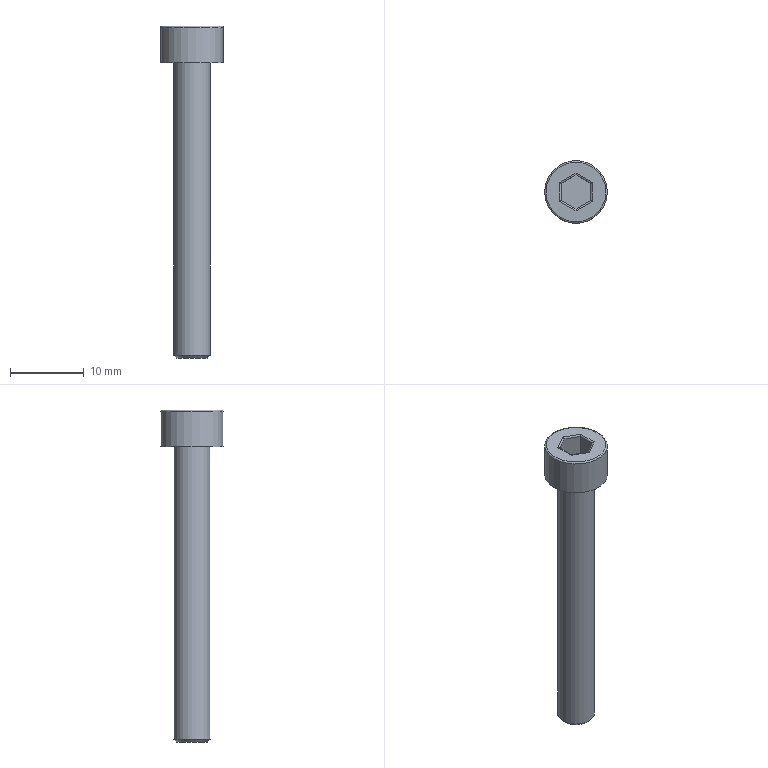Part | STEP file | 200 mesh_id694_x | 1 solid | 20 faces | box 8.5 x 8.5 x 45 mm | volume 1026 mm3 | plane 10 | cylinder 8 | torus 1 | cone 1 | commonest cylinder face diameters 0.4 x6 5 x1 8.5 x1
STEP:
#1=CARTESIAN_POINT('',(-17212.884,-3990.36,100.));
#2=VERTEX_POINT('',#1);
#3=CARTESIAN_POINT('',(-17215.084,-3989.089,100.));
#4=VERTEX_POINT('',#3);
#5=CARTESIAN_POINT('',(-17214.984,-3989.147,100.));
#6=DIRECTION('',(-0.866,0.5,0.));
#7=VECTOR('',#6,1.);
#8=LINE('',#5,#7);
#9=EDGE_CURVE('',#2,#4,#8,.T.);
#10=ORIENTED_EDGE('',*,*,#9,.T.);
#11=CARTESIAN_POINT('',(-17215.084,-3986.549,100.));
#12=VERTEX_POINT('',#11);
#13=CARTESIAN_POINT('',(-17215.084,-3986.664,100.));
#14=DIRECTION('',(0.,1.,0.));
#15=VECTOR('',#14,1.);
#16=LINE('',#13,#15);
#17=EDGE_CURVE('',#4,#12,#16,.T.);
#18=ORIENTED_EDGE('',*,*,#17,.T.);
#19=CARTESIAN_POINT('',(-17212.884,-3985.279,100.));
#20=VERTEX_POINT('',#19);
#21=CARTESIAN_POINT('',(-17212.984,-3985.337,100.));
#22=DIRECTION('',(0.866,0.5,0.));
#23=VECTOR('',#22,1.);
#24=LINE('',#21,#23);
#25=EDGE_CURVE('',#12,#20,#24,.T.);
#26=ORIENTED_EDGE('',*,*,#25,.T.);
#27=CARTESIAN_POINT('',(-17210.684,-3986.549,100.));
#28=VERTEX_POINT('',#27);
#29=CARTESIAN_POINT('',(-17210.784,-3986.491,100.));
#30=DIRECTION('',(0.866,-0.5,0.));
#31=VECTOR('',#30,1.);
#32=LINE('',#29,#31);
#33=EDGE_CURVE('',#20,#28,#32,.T.);
#34=ORIENTED_EDGE('',*,*,#33,.T.);
#35=CARTESIAN_POINT('',(-17210.684,-3989.089,100.));
#36=VERTEX_POINT('',#35);
#37=CARTESIAN_POINT('',(-17210.684,-3988.974,100.));
#38=DIRECTION('',(0.,-1.,0.));
#39=VECTOR('',#38,1.);
#40=LINE('',#37,#39);
#41=EDGE_CURVE('',#28,#36,#40,.T.);
#42=ORIENTED_EDGE('',*,*,#41,.T.);
#43=CARTESIAN_POINT('',(-17212.784,-3990.302,100.));
#44=DIRECTION('',(-0.866,-0.5,0.));
#45=VECTOR('',#44,1.);
#46=LINE('',#43,#45);
#47=EDGE_CURVE('',#36,#2,#46,.T.);
#48=ORIENTED_EDGE('',*,*,#47,.T.);
#49=EDGE_LOOP('',(#10,#18,#26,#34,#42,#48));
#50=FACE_BOUND('',#49,.T.);
#51=CARTESIAN_POINT('',(-17208.834,-3987.819,100.));
#52=VERTEX_POINT('',#51);
#53=CARTESIAN_POINT('',(-17212.884,-3987.819,100.));
#54=DIRECTION('',(0.,0.,1.));
#55=DIRECTION('',(1.,0.,0.));
#56=AXIS2_PLACEMENT_3D('',#53,#54,#55);
#57=CIRCLE('',#56,4.05);
#58=EDGE_CURVE('',#52,#52,#57,.T.);
#59=ORIENTED_EDGE('',*,*,#58,.T.);
#60=EDGE_LOOP('',(#59));
#61=FACE_BOUND('',#60,.T.);
#62=CARTESIAN_POINT('',(-17212.884,-3987.819,100.));
#63=DIRECTION('',(0.,0.,1.));
#64=DIRECTION('',(1.,0.,0.));
#65=AXIS2_PLACEMENT_3D('',#62,#63,#64);
#66=PLANE('',#65);
#67=ADVANCED_FACE('',(#50,#61),#66,.T.);
#68=CARTESIAN_POINT('',(-17215.384,-3987.819,95.));
#69=VERTEX_POINT('',#68);
#70=CARTESIAN_POINT('',(-17212.884,-3987.819,95.));
#71=DIRECTION('',(0.,0.,1.));
#72=DIRECTION('',(-1.,0.,0.));
#73=AXIS2_PLACEMENT_3D('',#70,#71,#72);
#74=CIRCLE('',#73,2.5);
#75=EDGE_CURVE('',#69,#69,#74,.T.);
#76=ORIENTED_EDGE('',*,*,#75,.T.);
#77=EDGE_LOOP('',(#76));
#78=FACE_BOUND('',#77,.T.);
#79=CARTESIAN_POINT('',(-17208.634,-3987.819,95.));
#80=VERTEX_POINT('',#79);
#81=CARTESIAN_POINT('',(-17212.884,-3987.819,95.));
#82=DIRECTION('',(0.,0.,1.));
#83=DIRECTION('',(1.,0.,0.));
#84=AXIS2_PLACEMENT_3D('',#81,#82,#83);
#85=CIRCLE('',#84,4.25);
#86=EDGE_CURVE('',#80,#80,#85,.T.);
#87=ORIENTED_EDGE('',*,*,#86,.F.);
#88=EDGE_LOOP('',(#87));
#89=FACE_BOUND('',#88,.T.);
#90=CARTESIAN_POINT('',(-17212.884,-3987.819,95.));
#91=DIRECTION('',(0.,0.,-1.));
#92=DIRECTION('',(-1.,0.,0.));
#93=AXIS2_PLACEMENT_3D('',#90,#91,#92);
#94=PLANE('',#93);
#95=ADVANCED_FACE('',(#78,#89),#94,.T.);
#96=CARTESIAN_POINT('',(-17208.634,-3987.819,99.8));
#97=VERTEX_POINT('',#96);
#98=CARTESIAN_POINT('',(-17212.884,-3987.819,99.8));
#99=DIRECTION('',(0.,0.,-1.));
#100=DIRECTION('',(1.,0.,0.));
#101=AXIS2_PLACEMENT_3D('',#98,#99,#100);
#102=CIRCLE('',#101,4.25);
#103=EDGE_CURVE('',#97,#97,#102,.T.);
#104=ORIENTED_EDGE('',*,*,#103,.T.);
#105=EDGE_LOOP('',(#104));
#106=FACE_BOUND('',#105,.T.);
#107=ORIENTED_EDGE('',*,*,#86,.T.);
#108=EDGE_LOOP('',(#107));
#109=FACE_BOUND('',#108,.T.);
#110=CARTESIAN_POINT('',(-17212.884,-3987.819,95.));
#111=DIRECTION('',(0.,0.,1.));
#112=DIRECTION('',(1.,0.,0.));
#113=AXIS2_PLACEMENT_3D('',#110,#111,#112);
#114=CYLINDRICAL_SURFACE('',#113,4.25);
#115=ADVANCED_FACE('',(#106,#109),#114,.T.);
#116=ORIENTED_EDGE('',*,*,#58,.F.);
#117=EDGE_LOOP('',(#116));
#118=FACE_BOUND('',#117,.T.);
#119=ORIENTED_EDGE('',*,*,#103,.F.);
#120=EDGE_LOOP('',(#119));
#121=FACE_BOUND('',#120,.T.);
#122=CARTESIAN_POINT('',(-17212.884,-3987.819,99.8));
#123=DIRECTION('',(0.,0.,1.));
#124=DIRECTION('',(1.,0.,0.));
#125=AXIS2_PLACEMENT_3D('',#122,#123,#124);
#126=TOROIDAL_SURFACE('',#125,4.05,0.2);
#127=ADVANCED_FACE('',(#118,#121),#126,.T.);
#128=CARTESIAN_POINT('',(-17212.884,-3985.51,99.8));
#129=VERTEX_POINT('',#128);
#130=CARTESIAN_POINT('',(-17212.884,-3985.51,97.));
#131=VERTEX_POINT('',#130);
#132=CARTESIAN_POINT('',(-17212.884,-3985.51,97.));
#133=DIRECTION('',(0.,0.,-1.));
#134=VECTOR('',#133,1.);
#135=LINE('',#132,#134);
#136=EDGE_CURVE('',#129,#131,#135,.T.);
#137=ORIENTED_EDGE('',*,*,#136,.F.);
#138=CARTESIAN_POINT('',(-17214.884,-3986.664,99.8));
#139=VERTEX_POINT('',#138);
#140=CARTESIAN_POINT('',(-17214.884,-3986.664,99.8));
#141=DIRECTION('',(-0.866,-0.5,0.));
#142=VECTOR('',#141,1.);
#143=LINE('',#140,#142);
#144=EDGE_CURVE('',#129,#139,#143,.T.);
#145=ORIENTED_EDGE('',*,*,#144,.T.);
#146=CARTESIAN_POINT('',(-17214.884,-3986.664,97.));
#147=VERTEX_POINT('',#146);
#148=CARTESIAN_POINT('',(-17214.884,-3986.664,97.));
#149=DIRECTION('',(0.,0.,-1.));
#150=VECTOR('',#149,1.);
#151=LINE('',#148,#150);
#152=EDGE_CURVE('',#139,#147,#151,.T.);
#153=ORIENTED_EDGE('',*,*,#152,.T.);
#154=CARTESIAN_POINT('',(-17212.884,-3985.51,97.));
#155=DIRECTION('',(0.866,0.5,0.));
#156=VECTOR('',#155,1.);
#157=LINE('',#154,#156);
#158=EDGE_CURVE('',#147,#131,#157,.T.);
#159=ORIENTED_EDGE('',*,*,#158,.T.);
#160=EDGE_LOOP('',(#137,#145,#153,#159));
#161=FACE_OUTER_BOUND('',#160,.T.);
#162=CARTESIAN_POINT('',(-17212.884,-3985.51,97.));
#163=DIRECTION('',(-0.5,0.866,0.));
#164=DIRECTION('',(-0.866,-0.5,0.));
#165=AXIS2_PLACEMENT_3D('',#162,#163,#164);
#166=PLANE('',#165);
#167=ADVANCED_FACE('',(#161),#166,.F.);
#168=ORIENTED_EDGE('',*,*,#152,.F.);
#169=CARTESIAN_POINT('',(-17214.884,-3988.974,99.8));
#170=VERTEX_POINT('',#169);
#171=CARTESIAN_POINT('',(-17214.884,-3988.974,99.8));
#172=DIRECTION('',(0.,-1.,0.));
#173=VECTOR('',#172,1.);
#174=LINE('',#171,#173);
#175=EDGE_CURVE('',#139,#170,#174,.T.);
#176=ORIENTED_EDGE('',*,*,#175,.T.);
#177=CARTESIAN_POINT('',(-17214.884,-3988.974,97.));
#178=VERTEX_POINT('',#177);
#179=CARTESIAN_POINT('',(-17214.884,-3988.974,97.));
#180=DIRECTION('',(0.,0.,-1.));
#181=VECTOR('',#180,1.);
#182=LINE('',#179,#181);
#183=EDGE_CURVE('',#170,#178,#182,.T.);
#184=ORIENTED_EDGE('',*,*,#183,.T.);
#185=CARTESIAN_POINT('',(-17214.884,-3986.664,97.));
#186=DIRECTION('',(0.,1.,0.));
#187=VECTOR('',#186,1.);
#188=LINE('',#185,#187);
#189=EDGE_CURVE('',#178,#147,#188,.T.);
#190=ORIENTED_EDGE('',*,*,#189,.T.);
#191=EDGE_LOOP('',(#168,#176,#184,#190));
#192=FACE_OUTER_BOUND('',#191,.T.);
#193=CARTESIAN_POINT('',(-17214.884,-3986.664,97.));
#194=DIRECTION('',(-1.,0.,0.));
#195=DIRECTION('',(0.,0.,1.));
#196=AXIS2_PLACEMENT_3D('',#193,#194,#195);
#197=PLANE('',#196);
#198=ADVANCED_FACE('',(#192),#197,.F.);
#199=ORIENTED_EDGE('',*,*,#183,.F.);
#200=CARTESIAN_POINT('',(-17212.884,-3990.129,99.8));
#201=VERTEX_POINT('',#200);
#202=CARTESIAN_POINT('',(-17212.884,-3990.129,99.8));
#203=DIRECTION('',(0.866,-0.5,0.));
#204=VECTOR('',#203,1.);
#205=LINE('',#202,#204);
#206=EDGE_CURVE('',#170,#201,#205,.T.);
#207=ORIENTED_EDGE('',*,*,#206,.T.);
#208=CARTESIAN_POINT('',(-17212.884,-3990.129,97.));
#209=VERTEX_POINT('',#208);
#210=CARTESIAN_POINT('',(-17212.884,-3990.129,97.));
#211=DIRECTION('',(0.,0.,-1.));
#212=VECTOR('',#211,1.);
#213=LINE('',#210,#212);
#214=EDGE_CURVE('',#201,#209,#213,.T.);
#215=ORIENTED_EDGE('',*,*,#214,.T.);
#216=CARTESIAN_POINT('',(-17214.884,-3988.974,97.));
#217=DIRECTION('',(-0.866,0.5,0.));
#218=VECTOR('',#217,1.);
#219=LINE('',#216,#218);
#220=EDGE_CURVE('',#209,#178,#219,.T.);
#221=ORIENTED_EDGE('',*,*,#220,.T.);
#222=EDGE_LOOP('',(#199,#207,#215,#221));
#223=FACE_OUTER_BOUND('',#222,.T.);
#224=CARTESIAN_POINT('',(-17214.884,-3988.974,97.));
#225=DIRECTION('',(-0.5,-0.866,0.));
#226=DIRECTION('',(0.866,-0.5,0.));
#227=AXIS2_PLACEMENT_3D('',#224,#225,#226);
#228=PLANE('',#227);
#229=ADVANCED_FACE('',(#223),#228,.F.);
#230=ORIENTED_EDGE('',*,*,#214,.F.);
#231=CARTESIAN_POINT('',(-17210.884,-3988.974,99.8));
#232=VERTEX_POINT('',#231);
#233=CARTESIAN_POINT('',(-17210.884,-3988.974,99.8));
#234=DIRECTION('',(0.866,0.5,0.));
#235=VECTOR('',#234,1.);
#236=LINE('',#233,#235);
#237=EDGE_CURVE('',#201,#232,#236,.T.);
#238=ORIENTED_EDGE('',*,*,#237,.T.);
#239=CARTESIAN_POINT('',(-17210.884,-3988.974,97.));
#240=VERTEX_POINT('',#239);
#241=CARTESIAN_POINT('',(-17210.884,-3988.974,97.));
#242=DIRECTION('',(0.,0.,-1.));
#243=VECTOR('',#242,1.);
#244=LINE('',#241,#243);
#245=EDGE_CURVE('',#232,#240,#244,.T.);
#246=ORIENTED_EDGE('',*,*,#245,.T.);
#247=CARTESIAN_POINT('',(-17212.884,-3990.129,97.));
#248=DIRECTION('',(-0.866,-0.5,0.));
#249=VECTOR('',#248,1.);
#250=LINE('',#247,#249);
#251=EDGE_CURVE('',#240,#209,#250,.T.);
#252=ORIENTED_EDGE('',*,*,#251,.T.);
#253=EDGE_LOOP('',(#230,#238,#246,#252));
#254=FACE_OUTER_BOUND('',#253,.T.);
#255=CARTESIAN_POINT('',(-17212.884,-3990.129,97.));
#256=DIRECTION('',(0.5,-0.866,0.));
#257=DIRECTION('',(0.866,0.5,0.));
#258=AXIS2_PLACEMENT_3D('',#255,#256,#257);
#259=PLANE('',#258);
#260=ADVANCED_FACE('',(#254),#259,.F.);
#261=ORIENTED_EDGE('',*,*,#245,.F.);
#262=CARTESIAN_POINT('',(-17210.884,-3986.664,99.8));
#263=VERTEX_POINT('',#262);
#264=CARTESIAN_POINT('',(-17210.884,-3986.664,99.8));
#265=DIRECTION('',(0.,1.,0.));
#266=VECTOR('',#265,1.);
#267=LINE('',#264,#266);
#268=EDGE_CURVE('',#232,#263,#267,.T.);
#269=ORIENTED_EDGE('',*,*,#268,.T.);
#270=CARTESIAN_POINT('',(-17210.884,-3986.664,97.));
#271=VERTEX_POINT('',#270);
#272=CARTESIAN_POINT('',(-17210.884,-3986.664,97.));
#273=DIRECTION('',(0.,0.,-1.));
#274=VECTOR('',#273,1.);
#275=LINE('',#272,#274);
#276=EDGE_CURVE('',#263,#271,#275,.T.);
#277=ORIENTED_EDGE('',*,*,#276,.T.);
#278=CARTESIAN_POINT('',(-17210.884,-3988.974,97.));
#279=DIRECTION('',(0.,-1.,0.));
#280=VECTOR('',#279,1.);
#281=LINE('',#278,#280);
#282=EDGE_CURVE('',#271,#240,#281,.T.);
#283=ORIENTED_EDGE('',*,*,#282,.T.);
#284=EDGE_LOOP('',(#261,#269,#277,#283));
#285=FACE_OUTER_BOUND('',#284,.T.);
#286=CARTESIAN_POINT('',(-17210.884,-3988.974,97.));
#287=DIRECTION('',(1.,0.,0.));
#288=DIRECTION('',(0.,0.,-1.));
#289=AXIS2_PLACEMENT_3D('',#286,#287,#288);
#290=PLANE('',#289);
#291=ADVANCED_FACE('',(#285),#290,.F.);
#292=ORIENTED_EDGE('',*,*,#276,.F.);
#293=CARTESIAN_POINT('',(-17212.884,-3985.51,99.8));
#294=DIRECTION('',(-0.866,0.5,0.));
#295=VECTOR('',#294,1.);
#296=LINE('',#293,#295);
#297=EDGE_CURVE('',#263,#129,#296,.T.);
#298=ORIENTED_EDGE('',*,*,#297,.T.);
#299=ORIENTED_EDGE('',*,*,#136,.T.);
#300=CARTESIAN_POINT('',(-17210.884,-3986.664,97.));
#301=DIRECTION('',(0.866,-0.5,0.));
#302=VECTOR('',#301,1.);
#303=LINE('',#300,#302);
#304=EDGE_CURVE('',#131,#271,#303,.T.);
#305=ORIENTED_EDGE('',*,*,#304,.T.);
#306=EDGE_LOOP('',(#292,#298,#299,#305));
#307=FACE_OUTER_BOUND('',#306,.T.);
#308=CARTESIAN_POINT('',(-17210.884,-3986.664,97.));
#309=DIRECTION('',(0.5,0.866,0.));
#310=DIRECTION('',(-0.866,0.5,0.));
#311=AXIS2_PLACEMENT_3D('',#308,#309,#310);
#312=PLANE('',#311);
#313=ADVANCED_FACE('',(#307),#312,.F.);
#314=ORIENTED_EDGE('',*,*,#158,.F.);
#315=ORIENTED_EDGE('',*,*,#189,.F.);
#316=ORIENTED_EDGE('',*,*,#220,.F.);
#317=ORIENTED_EDGE('',*,*,#251,.F.);
#318=ORIENTED_EDGE('',*,*,#282,.F.);
#319=ORIENTED_EDGE('',*,*,#304,.F.);
#320=EDGE_LOOP('',(#314,#315,#316,#317,#318,#319));
#321=FACE_OUTER_BOUND('',#320,.T.);
#322=CARTESIAN_POINT('',(-35.,70.,97.));
#323=DIRECTION('',(0.,0.,1.));
#324=DIRECTION('',(1.,0.,0.));
#325=AXIS2_PLACEMENT_3D('',#322,#323,#324);
#326=PLANE('',#325);
#327=ADVANCED_FACE('',(#321),#326,.T.);
#328=CARTESIAN_POINT('',(-17210.684,-3989.089,99.8));
#329=DIRECTION('',(-0.5,-0.866,0.));
#330=DIRECTION('',(0.866,-0.5,0.));
#331=AXIS2_PLACEMENT_3D('',#328,#329,#330);
#332=ELLIPSE('',#331,0.2309,0.2);
#333=EDGE_CURVE('',#36,#232,#332,.T.);
#334=ORIENTED_EDGE('',*,*,#333,.F.);
#335=ORIENTED_EDGE('',*,*,#41,.F.);
#336=CARTESIAN_POINT('',(-17210.684,-3986.549,99.8));
#337=DIRECTION('',(-0.5,0.866,0.));
#338=DIRECTION('',(0.866,0.5,0.));
#339=AXIS2_PLACEMENT_3D('',#336,#337,#338);
#340=ELLIPSE('',#339,0.2309,0.2);
#341=EDGE_CURVE('',#263,#28,#340,.T.);
#342=ORIENTED_EDGE('',*,*,#341,.F.);
#343=ORIENTED_EDGE('',*,*,#268,.F.);
#344=EDGE_LOOP('',(#334,#335,#342,#343));
#345=FACE_OUTER_BOUND('',#344,.T.);
#346=CARTESIAN_POINT('',(-17210.684,-3988.974,99.8));
#347=DIRECTION('',(0.,-1.,0.));
#348=DIRECTION('',(0.,0.,-1.));
#349=AXIS2_PLACEMENT_3D('',#346,#347,#348);
#350=CYLINDRICAL_SURFACE('',#349,0.2);
#351=ADVANCED_FACE('',(#345),#350,.T.);
#352=ORIENTED_EDGE('',*,*,#341,.T.);
#353=ORIENTED_EDGE('',*,*,#33,.F.);
#354=CARTESIAN_POINT('',(-17212.884,-3985.279,99.8));
#355=DIRECTION('',(-1.,0.,0.));
#356=DIRECTION('',(0.,1.,0.));
#357=AXIS2_PLACEMENT_3D('',#354,#355,#356);
#358=ELLIPSE('',#357,0.2309,0.2);
#359=EDGE_CURVE('',#129,#20,#358,.T.);
#360=ORIENTED_EDGE('',*,*,#359,.F.);
#361=ORIENTED_EDGE('',*,*,#297,.F.);
#362=EDGE_LOOP('',(#352,#353,#360,#361));
#363=FACE_OUTER_BOUND('',#362,.T.);
#364=CARTESIAN_POINT('',(-17210.784,-3986.491,99.8));
#365=DIRECTION('',(0.866,-0.5,0.));
#366=DIRECTION('',(0.5,0.866,0.));
#367=AXIS2_PLACEMENT_3D('',#364,#365,#366);
#368=CYLINDRICAL_SURFACE('',#367,0.2);
#369=ADVANCED_FACE('',(#363),#368,.T.);
#370=ORIENTED_EDGE('',*,*,#333,.T.);
#371=ORIENTED_EDGE('',*,*,#237,.F.);
#372=CARTESIAN_POINT('',(-17212.884,-3990.36,99.8));
#373=DIRECTION('',(-1.,0.,0.));
#374=DIRECTION('',(0.,-1.,0.));
#375=AXIS2_PLACEMENT_3D('',#372,#373,#374);
#376=ELLIPSE('',#375,0.2309,0.2);
#377=EDGE_CURVE('',#2,#201,#376,.T.);
#378=ORIENTED_EDGE('',*,*,#377,.F.);
#379=ORIENTED_EDGE('',*,*,#47,.F.);
#380=EDGE_LOOP('',(#370,#371,#378,#379));
#381=FACE_OUTER_BOUND('',#380,.T.);
#382=CARTESIAN_POINT('',(-17212.784,-3990.302,99.8));
#383=DIRECTION('',(-0.866,-0.5,0.));
#384=DIRECTION('',(0.5,-0.866,0.));
#385=AXIS2_PLACEMENT_3D('',#382,#383,#384);
#386=CYLINDRICAL_SURFACE('',#385,0.2);
#387=ADVANCED_FACE('',(#381),#386,.T.);
#388=ORIENTED_EDGE('',*,*,#359,.T.);
#389=ORIENTED_EDGE('',*,*,#25,.F.);
#390=CARTESIAN_POINT('',(-17215.084,-3986.549,99.8));
#391=DIRECTION('',(-0.5,-0.866,0.));
#392=DIRECTION('',(-0.866,0.5,0.));
#393=AXIS2_PLACEMENT_3D('',#390,#391,#392);
#394=ELLIPSE('',#393,0.2309,0.2);
#395=EDGE_CURVE('',#139,#12,#394,.T.);
#396=ORIENTED_EDGE('',*,*,#395,.F.);
#397=ORIENTED_EDGE('',*,*,#144,.F.);
#398=EDGE_LOOP('',(#388,#389,#396,#397));
#399=FACE_OUTER_BOUND('',#398,.T.);
#400=CARTESIAN_POINT('',(-17212.984,-3985.337,99.8));
#401=DIRECTION('',(0.866,0.5,0.));
#402=DIRECTION('',(-0.5,0.866,0.));
#403=AXIS2_PLACEMENT_3D('',#400,#401,#402);
#404=CYLINDRICAL_SURFACE('',#403,0.2);
#405=ADVANCED_FACE('',(#399),#404,.T.);
#406=ORIENTED_EDGE('',*,*,#377,.T.);
#407=ORIENTED_EDGE('',*,*,#206,.F.);
#408=CARTESIAN_POINT('',(-17215.084,-3989.089,99.8));
#409=DIRECTION('',(-0.5,0.866,0.));
#410=DIRECTION('',(0.866,0.5,0.));
#411=AXIS2_PLACEMENT_3D('',#408,#409,#410);
#412=ELLIPSE('',#411,0.2309,0.2);
#413=EDGE_CURVE('',#4,#170,#412,.T.);
#414=ORIENTED_EDGE('',*,*,#413,.F.);
#415=ORIENTED_EDGE('',*,*,#9,.F.);
#416=EDGE_LOOP('',(#406,#407,#414,#415));
#417=FACE_OUTER_BOUND('',#416,.T.);
#418=CARTESIAN_POINT('',(-17214.984,-3989.147,99.8));
#419=DIRECTION('',(-0.866,0.5,0.));
#420=DIRECTION('',(-0.5,-0.866,0.));
#421=AXIS2_PLACEMENT_3D('',#418,#419,#420);
#422=CYLINDRICAL_SURFACE('',#421,0.2);
#423=ADVANCED_FACE('',(#417),#422,.T.);
#424=ORIENTED_EDGE('',*,*,#395,.T.);
#425=ORIENTED_EDGE('',*,*,#17,.F.);
#426=ORIENTED_EDGE('',*,*,#413,.T.);
#427=ORIENTED_EDGE('',*,*,#175,.F.);
#428=EDGE_LOOP('',(#424,#425,#426,#427));
#429=FACE_OUTER_BOUND('',#428,.T.);
#430=CARTESIAN_POINT('',(-17215.084,-3986.664,99.8));
#431=DIRECTION('',(0.,1.,0.));
#432=DIRECTION('',(0.,0.,1.));
#433=AXIS2_PLACEMENT_3D('',#430,#431,#432);
#434=CYLINDRICAL_SURFACE('',#433,0.2);
#435=ADVANCED_FACE('',(#429),#434,.T.);
#436=CARTESIAN_POINT('',(-17215.384,-3987.819,55.4));
#437=VERTEX_POINT('',#436);
#438=CARTESIAN_POINT('',(-17212.884,-3987.819,55.4));
#439=DIRECTION('',(0.,0.,1.));
#440=DIRECTION('',(-1.,0.,0.));
#441=AXIS2_PLACEMENT_3D('',#438,#439,#440);
#442=CIRCLE('',#441,2.5);
#443=EDGE_CURVE('',#437,#437,#442,.T.);
#444=ORIENTED_EDGE('',*,*,#443,.T.);
#445=EDGE_LOOP('',(#444));
#446=FACE_BOUND('',#445,.T.);
#447=ORIENTED_EDGE('',*,*,#75,.F.);
#448=EDGE_LOOP('',(#447));
#449=FACE_BOUND('',#448,.T.);
#450=CARTESIAN_POINT('',(-17212.884,-3987.819,92.));
#451=DIRECTION('',(0.,0.,-1.));
#452=DIRECTION('',(1.,0.,0.));
#453=AXIS2_PLACEMENT_3D('',#450,#451,#452);
#454=CYLINDRICAL_SURFACE('',#453,2.5);
#455=ADVANCED_FACE('',(#446,#449),#454,.T.);
#456=CARTESIAN_POINT('',(-17214.984,-3987.819,55.));
#457=VERTEX_POINT('',#456);
#458=CARTESIAN_POINT('',(-17212.884,-3987.819,55.));
#459=DIRECTION('',(0.,0.,-1.));
#460=DIRECTION('',(-1.,0.,0.));
#461=AXIS2_PLACEMENT_3D('',#458,#459,#460);
#462=CIRCLE('',#461,2.1);
#463=EDGE_CURVE('',#457,#457,#462,.T.);
#464=ORIENTED_EDGE('',*,*,#463,.T.);
#465=EDGE_LOOP('',(#464));
#466=FACE_OUTER_BOUND('',#465,.T.);
#467=CARTESIAN_POINT('',(-17212.884,-3987.819,55.));
#468=DIRECTION('',(0.,0.,-1.));
#469=DIRECTION('',(-1.,0.,0.));
#470=AXIS2_PLACEMENT_3D('',#467,#468,#469);
#471=PLANE('',#470);
#472=ADVANCED_FACE('',(#466),#471,.T.);
#473=ORIENTED_EDGE('',*,*,#463,.F.);
#474=EDGE_LOOP('',(#473));
#475=FACE_BOUND('',#474,.T.);
#476=ORIENTED_EDGE('',*,*,#443,.F.);
#477=EDGE_LOOP('',(#476));
#478=FACE_BOUND('',#477,.T.);
#479=CARTESIAN_POINT('',(-17212.884,-3987.819,55.4));
#480=DIRECTION('',(0.,0.,1.));
#481=DIRECTION('',(1.,0.,0.));
#482=AXIS2_PLACEMENT_3D('',#479,#480,#481);
#483=CONICAL_SURFACE('',#482,2.5,45.);
#484=ADVANCED_FACE('',(#475,#478),#483,.T.);
#485=CLOSED_SHELL('',(#67,#95,#115,#127,#167,#198,#229,#260,#291,#313,#327,#351,#369,#387,#405,#423,#435,#455,#472,#484));
#486=MANIFOLD_SOLID_BREP('',#485);
#487=(LENGTH_UNIT()NAMED_UNIT(*)SI_UNIT(.MILLI.,.METRE.));
#488=UNCERTAINTY_MEASURE_WITH_UNIT(LENGTH_MEASURE(0.00002),#487,'','');
#489=(NAMED_UNIT(*)PLANE_ANGLE_UNIT()SI_UNIT($,.RADIAN.));
#490=PLANE_ANGLE_MEASURE_WITH_UNIT(PLANE_ANGLE_MEASURE(0.01745),#489);
#491=DIMENSIONAL_EXPONENTS(0.,0.,0.,0.,0.,0.,0.);
#492=(CONVERSION_BASED_UNIT('DEGREE',#490)NAMED_UNIT(#491)PLANE_ANGLE_UNIT());
#493=(NAMED_UNIT(*)SI_UNIT($,.STERADIAN.)SOLID_ANGLE_UNIT());
#494=(GEOMETRIC_REPRESENTATION_CONTEXT(3)GLOBAL_UNCERTAINTY_ASSIGNED_CONTEXT((#488))GLOBAL_UNIT_ASSIGNED_CONTEXT((#487,#492,#493))REPRESENTATION_CONTEXT('',''));
#495=ADVANCED_BREP_SHAPE_REPRESENTATION('',(#486),#494);